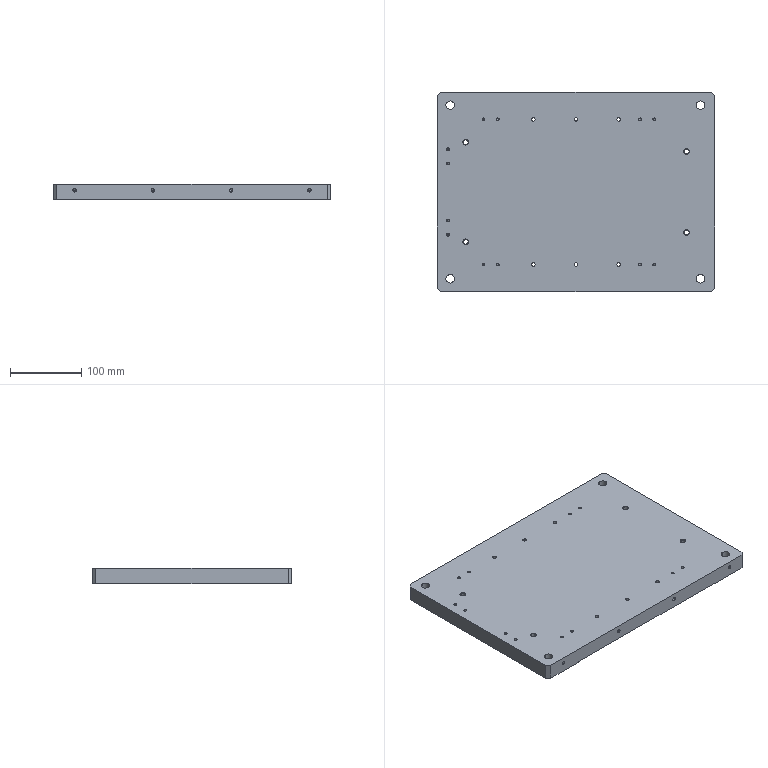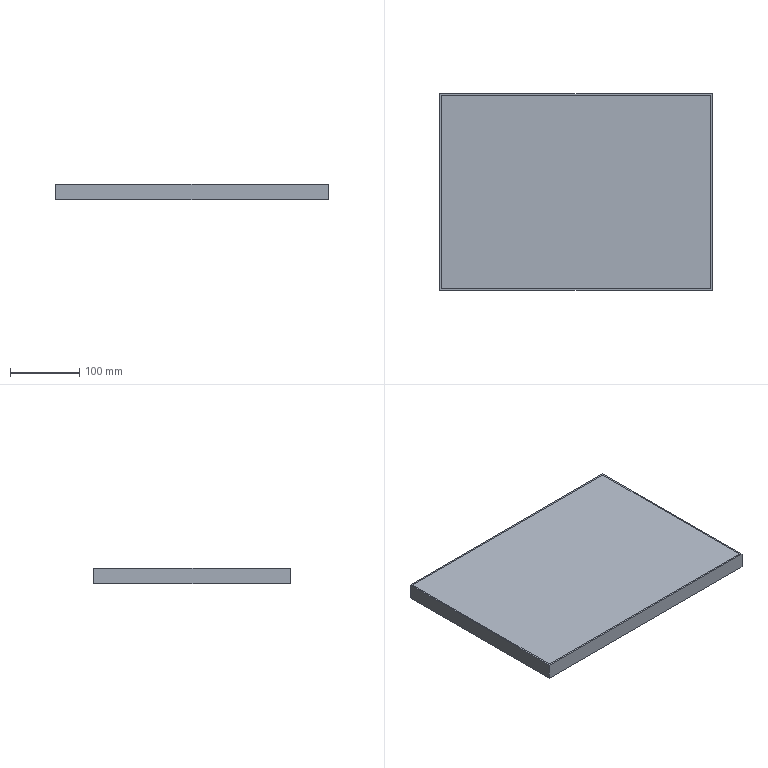CAM job | NX | 3-axis milling, drilling | part box 390 x 280 x 22 mm | stock box 395 x 285 x 23 mm
Tools:
number,name,description,diameter,corner_radius,flute_length,length,flutes
1,D20R0.8,Milling Tool-5 Parameters,20.0,0.8,50.0,75.0,2
6,D6,Milling Tool-5 Parameters,6.0,0.0,50.0,75.0,2
2,D10,Milling Tool-5 Parameters,10.0,0.0,50.0,75.0,2
7,D6A45,Milling Tool-5 Parameters,6.0,0.0,50.0,75.0,2
10,3.3ZT,Drilling Tool,3.3,0.0,35.0,50.0,2
Operations:
program,operation,operation_type,tool,method,geometry_group,spindle_rpm,surface_speed,feed_per_tooth,feed_cut,feed_plunge,cut_length_mm,path_length_mm,cut_time_min,machine_time_min
1,FLOOR_WALL,VolumeBased25DMillingOperation,D20R0.8,METHOD,A,7500.0,471.0,0.09,1350.0,100.0,12324.638,12378.638,9.129,9.135
1,ZLEVEL_PROFILE_1,ZLevelMilling,D6,METHOD,A,9500.0,179.0,0.1579,3000.0,1000.0,99787.41,99866.36,33.285,33.293
1,ZLEVEL_PROFILE_COPY,ZLevelMilling,D6,METHOD,A,9500.0,179.0,0.0789,1500.0,1000.0,3326.86,3416.785,2.219,2.228
1,HOLE_MILLING,CylinderMilling,D6,METHOD,A,9500.0,179.0,0.0842,1600.0,100.0,5756.112,6921.912,3.598,3.714
1,DRILLING,Operation,D6A45,METHOD,A,5000.0,94.0,0.025,250.0,0.0,88.0,1164.928,0.352,0.4597
1,DRILLING_COPY_COPY,Operation,3.3ZT,METHOD,A,2000.0,20.0,0.0375,150.0,0.0,167.897,1160.974,1.119,1.219
1,PLANAR_MILL,PlanarMilling,D6A45,METHOD,A,9500.0,179.0,0.0658,1250.0,500.0,1502.588,2639.012,1.226,1.34
2,FLOOR_WALL_COPY,VolumeBased25DMillingOperation,D20R0.8,METHOD,B,7500.0,471.0,0.09,1350.0,100.0,12174.639,12228.639,9.018,9.024
2,FLOOR_WALL_1,VolumeBased25DMillingOperation,D10,METHOD,B,9500.0,298.0,0.1316,2500.0,100.0,32135.991,32821.185,12.854,12.923
2,FLOOR_WALL_1_COPY,VolumeBased25DMillingOperation,D10,METHOD,B,9500.0,298.0,0.0711,1350.0,100.0,15641.999,15697.999,11.587,11.592
2,PLANAR_MILL_COPY,PlanarMilling,D6A45,METHOD,B,9500.0,179.0,0.0658,1250.0,500.0,1539.479,2765.328,1.261,1.383
2,PLANAR_MILL_COPY_COPY,PlanarMilling,D6A45,METHOD,B,9500.0,179.0,0.0658,1250.0,500.0,549.228,949.925,0.4505,0.4906